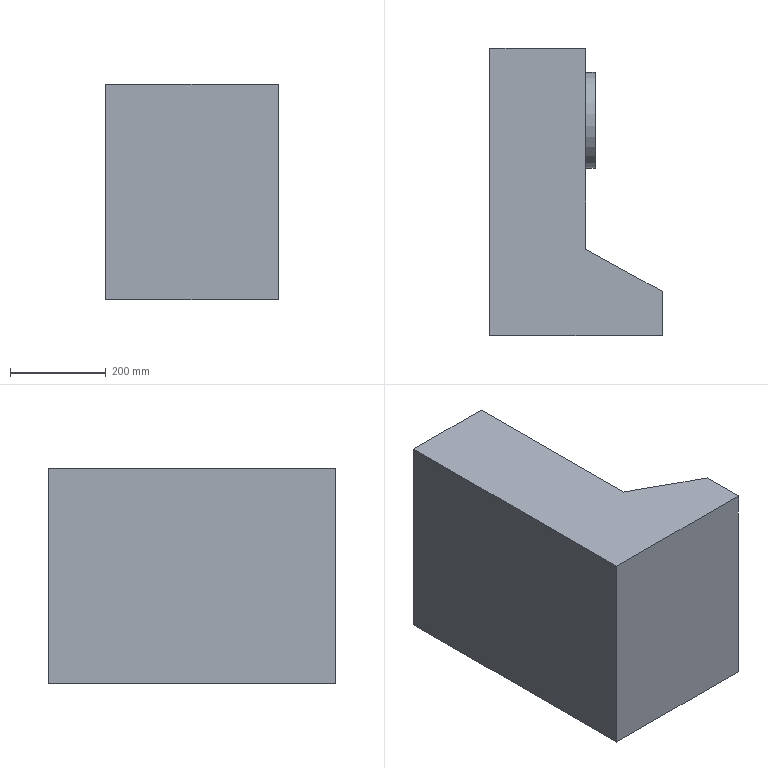Part | SolidWorks | features ICE 3, Extrusion 1 | 1 solid | 11 faces | box 360 x 600 x 450 mm | volume 64420319 mm3 | plane 9 | cylinder 2 | commonest cylinder face diameters 200 x2
STEP:
#1=CARTESIAN_POINT('',(220.,250.,0.));
#2=VERTEX_POINT('',#1);
#3=CARTESIAN_POINT('',(220.,50.,0.));
#4=VERTEX_POINT('',#3);
#5=CARTESIAN_POINT('',(220.,150.,0.));
#6=DIRECTION('',(1.,0.,0.));
#7=DIRECTION('',(0.,1.,0.));
#8=AXIS2_PLACEMENT_3D('',#5,#6,#7);
#9=CIRCLE('',#8,100.);
#10=EDGE_CURVE('',#2,#4,#9,.T.);
#11=ORIENTED_EDGE('',*,*,#10,.F.);
#12=CARTESIAN_POINT('',(200.,250.,0.));
#13=VERTEX_POINT('',#12);
#14=CARTESIAN_POINT('',(220.,250.,0.));
#15=DIRECTION('',(-1.,0.,0.));
#16=VECTOR('',#15,1000.);
#17=LINE('',#14,#16);
#18=EDGE_CURVE('',#2,#13,#17,.T.);
#19=ORIENTED_EDGE('',*,*,#18,.T.);
#20=CARTESIAN_POINT('',(200.,50.,0.));
#21=VERTEX_POINT('',#20);
#22=CARTESIAN_POINT('',(200.,150.,0.));
#23=DIRECTION('',(1.,0.,0.));
#24=DIRECTION('',(0.,-1.,0.));
#25=AXIS2_PLACEMENT_3D('',#22,#23,#24);
#26=CIRCLE('',#25,100.);
#27=EDGE_CURVE('',#13,#21,#26,.T.);
#28=ORIENTED_EDGE('',*,*,#27,.T.);
#29=CARTESIAN_POINT('',(220.,50.,0.));
#30=DIRECTION('',(-1.,0.,0.));
#31=VECTOR('',#30,1000.);
#32=LINE('',#29,#31);
#33=EDGE_CURVE('',#4,#21,#32,.T.);
#34=ORIENTED_EDGE('',*,*,#33,.F.);
#35=EDGE_LOOP('',(#11,#19,#28,#34));
#36=FACE_OUTER_BOUND('',#35,.T.);
#37=CARTESIAN_POINT('',(220.,150.,0.));
#38=DIRECTION('',(-1.,0.,0.));
#39=DIRECTION('',(0.,-1.,0.));
#40=AXIS2_PLACEMENT_3D('',#37,#38,#39);
#41=CYLINDRICAL_SURFACE('',#40,100.);
#42=ADVANCED_FACE('',(#36),#41,.T.);
#43=CARTESIAN_POINT('',(360.,-300.,-225.));
#44=VERTEX_POINT('',#43);
#45=CARTESIAN_POINT('',(360.,-208.,-225.));
#46=VERTEX_POINT('',#45);
#47=CARTESIAN_POINT('',(360.,300.,-225.));
#48=DIRECTION('',(0.,1.,0.));
#49=VECTOR('',#48,1000.);
#50=LINE('',#47,#49);
#51=EDGE_CURVE('',#44,#46,#50,.T.);
#52=ORIENTED_EDGE('',*,*,#51,.F.);
#53=CARTESIAN_POINT('',(0.,-300.,-225.));
#54=VERTEX_POINT('',#53);
#55=CARTESIAN_POINT('',(400.,-300.,-225.));
#56=DIRECTION('',(-1.,0.,0.));
#57=VECTOR('',#56,1000.);
#58=LINE('',#55,#57);
#59=EDGE_CURVE('',#44,#54,#58,.T.);
#60=ORIENTED_EDGE('',*,*,#59,.T.);
#61=CARTESIAN_POINT('',(0.,300.,-225.));
#62=VERTEX_POINT('',#61);
#63=CARTESIAN_POINT('',(0.,300.,-225.));
#64=DIRECTION('',(0.,1.,0.));
#65=VECTOR('',#64,1000.);
#66=LINE('',#63,#65);
#67=EDGE_CURVE('',#54,#62,#66,.T.);
#68=ORIENTED_EDGE('',*,*,#67,.T.);
#69=CARTESIAN_POINT('',(200.,300.,-225.));
#70=VERTEX_POINT('',#69);
#71=CARTESIAN_POINT('',(400.,300.,-225.));
#72=DIRECTION('',(-1.,0.,0.));
#73=VECTOR('',#72,1000.);
#74=LINE('',#71,#73);
#75=EDGE_CURVE('',#70,#62,#74,.T.);
#76=ORIENTED_EDGE('',*,*,#75,.F.);
#77=CARTESIAN_POINT('',(200.,-120.,-225.));
#78=VERTEX_POINT('',#77);
#79=CARTESIAN_POINT('',(200.,300.,-225.));
#80=DIRECTION('',(0.,-1.,0.));
#81=VECTOR('',#80,1000.);
#82=LINE('',#79,#81);
#83=EDGE_CURVE('',#70,#78,#82,.T.);
#84=ORIENTED_EDGE('',*,*,#83,.T.);
#85=CARTESIAN_POINT('',(176.2,-106.91,-225.));
#86=DIRECTION('',(0.8762,-0.4819,0.));
#87=VECTOR('',#86,1000.);
#88=LINE('',#85,#87);
#89=EDGE_CURVE('',#78,#46,#88,.T.);
#90=ORIENTED_EDGE('',*,*,#89,.T.);
#91=EDGE_LOOP('',(#52,#60,#68,#76,#84,#90));
#92=FACE_OUTER_BOUND('',#91,.T.);
#93=CARTESIAN_POINT('',(400.,300.,-225.));
#94=DIRECTION('',(0.,0.,1.));
#95=DIRECTION('',(1.,0.,0.));
#96=AXIS2_PLACEMENT_3D('',#93,#94,#95);
#97=PLANE('',#96);
#98=ADVANCED_FACE('',(#92),#97,.F.);
#99=CARTESIAN_POINT('',(360.,-208.,225.));
#100=VERTEX_POINT('',#99);
#101=CARTESIAN_POINT('',(360.,-300.,225.));
#102=VERTEX_POINT('',#101);
#103=CARTESIAN_POINT('',(360.,300.,225.));
#104=DIRECTION('',(0.,-1.,0.));
#105=VECTOR('',#104,1000.);
#106=LINE('',#103,#105);
#107=EDGE_CURVE('',#100,#102,#106,.T.);
#108=ORIENTED_EDGE('',*,*,#107,.F.);
#109=CARTESIAN_POINT('',(200.,-120.,225.));
#110=VERTEX_POINT('',#109);
#111=CARTESIAN_POINT('',(200.,-120.,225.));
#112=DIRECTION('',(0.8762,-0.4819,0.));
#113=VECTOR('',#112,1000.);
#114=LINE('',#111,#113);
#115=EDGE_CURVE('',#110,#100,#114,.T.);
#116=ORIENTED_EDGE('',*,*,#115,.F.);
#117=CARTESIAN_POINT('',(200.,300.,225.));
#118=VERTEX_POINT('',#117);
#119=CARTESIAN_POINT('',(200.,300.,225.));
#120=DIRECTION('',(0.,-1.,0.));
#121=VECTOR('',#120,1000.);
#122=LINE('',#119,#121);
#123=EDGE_CURVE('',#118,#110,#122,.T.);
#124=ORIENTED_EDGE('',*,*,#123,.F.);
#125=CARTESIAN_POINT('',(0.,300.,225.));
#126=VERTEX_POINT('',#125);
#127=CARTESIAN_POINT('',(400.,300.,225.));
#128=DIRECTION('',(-1.,0.,0.));
#129=VECTOR('',#128,1000.);
#130=LINE('',#127,#129);
#131=EDGE_CURVE('',#118,#126,#130,.T.);
#132=ORIENTED_EDGE('',*,*,#131,.T.);
#133=CARTESIAN_POINT('',(0.,-300.,225.));
#134=VERTEX_POINT('',#133);
#135=CARTESIAN_POINT('',(0.,300.,225.));
#136=DIRECTION('',(0.,-1.,0.));
#137=VECTOR('',#136,1000.);
#138=LINE('',#135,#137);
#139=EDGE_CURVE('',#126,#134,#138,.T.);
#140=ORIENTED_EDGE('',*,*,#139,.T.);
#141=CARTESIAN_POINT('',(400.,-300.,225.));
#142=DIRECTION('',(-1.,0.,0.));
#143=VECTOR('',#142,1000.);
#144=LINE('',#141,#143);
#145=EDGE_CURVE('',#102,#134,#144,.T.);
#146=ORIENTED_EDGE('',*,*,#145,.F.);
#147=EDGE_LOOP('',(#108,#116,#124,#132,#140,#146));
#148=FACE_OUTER_BOUND('',#147,.T.);
#149=CARTESIAN_POINT('',(400.,300.,225.));
#150=DIRECTION('',(0.,0.,-1.));
#151=DIRECTION('',(0.,1.,0.));
#152=AXIS2_PLACEMENT_3D('',#149,#150,#151);
#153=PLANE('',#152);
#154=ADVANCED_FACE('',(#148),#153,.F.);
#155=CARTESIAN_POINT('',(360.,-300.,225.));
#156=DIRECTION('',(0.,0.,-1.));
#157=VECTOR('',#156,1000.);
#158=LINE('',#155,#157);
#159=EDGE_CURVE('',#102,#44,#158,.T.);
#160=ORIENTED_EDGE('',*,*,#159,.F.);
#161=ORIENTED_EDGE('',*,*,#145,.T.);
#162=CARTESIAN_POINT('',(0.,-300.,225.));
#163=DIRECTION('',(0.,0.,-1.));
#164=VECTOR('',#163,1000.);
#165=LINE('',#162,#164);
#166=EDGE_CURVE('',#134,#54,#165,.T.);
#167=ORIENTED_EDGE('',*,*,#166,.T.);
#168=ORIENTED_EDGE('',*,*,#59,.F.);
#169=EDGE_LOOP('',(#160,#161,#167,#168));
#170=FACE_OUTER_BOUND('',#169,.T.);
#171=CARTESIAN_POINT('',(400.,-300.,225.));
#172=DIRECTION('',(0.,1.,0.));
#173=DIRECTION('',(0.,0.,1.));
#174=AXIS2_PLACEMENT_3D('',#171,#172,#173);
#175=PLANE('',#174);
#176=ADVANCED_FACE('',(#170),#175,.F.);
#177=CARTESIAN_POINT('',(360.,-208.,-2175.));
#178=DIRECTION('',(0.,0.,1.));
#179=VECTOR('',#178,1000.);
#180=LINE('',#177,#179);
#181=EDGE_CURVE('',#46,#100,#180,.T.);
#182=ORIENTED_EDGE('',*,*,#181,.F.);
#183=ORIENTED_EDGE('',*,*,#89,.F.);
#184=CARTESIAN_POINT('',(200.,-120.,-2175.));
#185=DIRECTION('',(0.,0.,1.));
#186=VECTOR('',#185,1000.);
#187=LINE('',#184,#186);
#188=EDGE_CURVE('',#78,#110,#187,.T.);
#189=ORIENTED_EDGE('',*,*,#188,.T.);
#190=ORIENTED_EDGE('',*,*,#115,.T.);
#191=EDGE_LOOP('',(#182,#183,#189,#190));
#192=FACE_OUTER_BOUND('',#191,.T.);
#193=CARTESIAN_POINT('',(200.,-120.,-2175.));
#194=DIRECTION('',(-0.4819,-0.8762,0.));
#195=DIRECTION('',(0.8762,-0.4819,0.));
#196=AXIS2_PLACEMENT_3D('',#193,#194,#195);
#197=PLANE('',#196);
#198=ADVANCED_FACE('',(#192),#197,.F.);
#199=ORIENTED_EDGE('',*,*,#131,.F.);
#200=CARTESIAN_POINT('',(200.,300.,-2175.));
#201=DIRECTION('',(0.,0.,1.));
#202=VECTOR('',#201,1000.);
#203=LINE('',#200,#202);
#204=EDGE_CURVE('',#70,#118,#203,.T.);
#205=ORIENTED_EDGE('',*,*,#204,.F.);
#206=ORIENTED_EDGE('',*,*,#75,.T.);
#207=CARTESIAN_POINT('',(0.,300.,225.));
#208=DIRECTION('',(0.,0.,1.));
#209=VECTOR('',#208,1000.);
#210=LINE('',#207,#209);
#211=EDGE_CURVE('',#62,#126,#210,.T.);
#212=ORIENTED_EDGE('',*,*,#211,.T.);
#213=EDGE_LOOP('',(#199,#205,#206,#212));
#214=FACE_OUTER_BOUND('',#213,.T.);
#215=CARTESIAN_POINT('',(400.,300.,225.));
#216=DIRECTION('',(0.,-1.,0.));
#217=DIRECTION('',(0.,0.,-1.));
#218=AXIS2_PLACEMENT_3D('',#215,#216,#217);
#219=PLANE('',#218);
#220=ADVANCED_FACE('',(#214),#219,.F.);
#221=ORIENTED_EDGE('',*,*,#67,.F.);
#222=ORIENTED_EDGE('',*,*,#166,.F.);
#223=ORIENTED_EDGE('',*,*,#139,.F.);
#224=ORIENTED_EDGE('',*,*,#211,.F.);
#225=EDGE_LOOP('',(#221,#222,#223,#224));
#226=FACE_OUTER_BOUND('',#225,.T.);
#227=CARTESIAN_POINT('',(0.,0.,0.));
#228=DIRECTION('',(1.,0.,0.));
#229=DIRECTION('',(0.,0.,-1.));
#230=AXIS2_PLACEMENT_3D('',#227,#228,#229);
#231=PLANE('',#230);
#232=ADVANCED_FACE('',(#226),#231,.F.);
#233=CARTESIAN_POINT('',(200.,150.,0.));
#234=DIRECTION('',(1.,0.,0.));
#235=DIRECTION('',(0.,-1.,0.));
#236=AXIS2_PLACEMENT_3D('',#233,#234,#235);
#237=CIRCLE('',#236,100.);
#238=EDGE_CURVE('',#21,#13,#237,.T.);
#239=ORIENTED_EDGE('',*,*,#238,.F.);
#240=ORIENTED_EDGE('',*,*,#27,.F.);
#241=EDGE_LOOP('',(#239,#240));
#242=FACE_BOUND('',#241,.T.);
#243=ORIENTED_EDGE('',*,*,#204,.T.);
#244=ORIENTED_EDGE('',*,*,#123,.T.);
#245=ORIENTED_EDGE('',*,*,#188,.F.);
#246=ORIENTED_EDGE('',*,*,#83,.F.);
#247=EDGE_LOOP('',(#243,#244,#245,#246));
#248=FACE_OUTER_BOUND('',#247,.T.);
#249=CARTESIAN_POINT('',(200.,300.,-2175.));
#250=DIRECTION('',(-1.,0.,0.));
#251=DIRECTION('',(0.,-1.,0.));
#252=AXIS2_PLACEMENT_3D('',#249,#250,#251);
#253=PLANE('',#252);
#254=ADVANCED_FACE('',(#242,#248),#253,.F.);
#255=ORIENTED_EDGE('',*,*,#159,.T.);
#256=ORIENTED_EDGE('',*,*,#51,.T.);
#257=ORIENTED_EDGE('',*,*,#181,.T.);
#258=ORIENTED_EDGE('',*,*,#107,.T.);
#259=EDGE_LOOP('',(#255,#256,#257,#258));
#260=FACE_OUTER_BOUND('',#259,.T.);
#261=CARTESIAN_POINT('',(360.,0.,0.));
#262=DIRECTION('',(1.,0.,0.));
#263=DIRECTION('',(0.,0.,-1.));
#264=AXIS2_PLACEMENT_3D('',#261,#262,#263);
#265=PLANE('',#264);
#266=ADVANCED_FACE('',(#260),#265,.T.);
#267=ORIENTED_EDGE('',*,*,#18,.F.);
#268=CARTESIAN_POINT('',(220.,150.,0.));
#269=DIRECTION('',(1.,0.,0.));
#270=DIRECTION('',(0.,1.,0.));
#271=AXIS2_PLACEMENT_3D('',#268,#269,#270);
#272=CIRCLE('',#271,100.);
#273=EDGE_CURVE('',#4,#2,#272,.T.);
#274=ORIENTED_EDGE('',*,*,#273,.F.);
#275=ORIENTED_EDGE('',*,*,#33,.T.);
#276=ORIENTED_EDGE('',*,*,#238,.T.);
#277=EDGE_LOOP('',(#267,#274,#275,#276));
#278=FACE_OUTER_BOUND('',#277,.T.);
#279=CARTESIAN_POINT('',(220.,150.,0.));
#280=DIRECTION('',(-1.,0.,0.));
#281=DIRECTION('',(0.,-1.,0.));
#282=AXIS2_PLACEMENT_3D('',#279,#280,#281);
#283=CYLINDRICAL_SURFACE('',#282,100.);
#284=ADVANCED_FACE('',(#278),#283,.T.);
#285=ORIENTED_EDGE('',*,*,#273,.T.);
#286=ORIENTED_EDGE('',*,*,#10,.T.);
#287=EDGE_LOOP('',(#285,#286));
#288=FACE_OUTER_BOUND('',#287,.T.);
#289=CARTESIAN_POINT('',(220.,150.,0.));
#290=DIRECTION('',(1.,0.,0.));
#291=DIRECTION('',(0.,1.,0.));
#292=AXIS2_PLACEMENT_3D('',#289,#290,#291);
#293=PLANE('',#292);
#294=ADVANCED_FACE('',(#288),#293,.T.);
#295=CLOSED_SHELL('',(#42,#98,#154,#176,#198,#220,#232,#254,#266,#284,#294));
#296=MANIFOLD_SOLID_BREP('',#295);
#297=CARTESIAN_POINT('',(0.,0.,0.));
#298=DIRECTION('',(0.,0.,1.));
#299=DIRECTION('',(1.,0.,0.));
#300=AXIS2_PLACEMENT_3D('',#297,#298,#299);
#301=(LENGTH_UNIT()NAMED_UNIT(*)SI_UNIT(.MILLI.,.METRE.));
#302=UNCERTAINTY_MEASURE_WITH_UNIT(LENGTH_MEASURE(0.00001),#301,'','');
#303=(NAMED_UNIT(*)PLANE_ANGLE_UNIT()SI_UNIT($,.RADIAN.));
#304=(NAMED_UNIT(*)SI_UNIT($,.STERADIAN.)SOLID_ANGLE_UNIT());
#305=(GEOMETRIC_REPRESENTATION_CONTEXT(3)GLOBAL_UNCERTAINTY_ASSIGNED_CONTEXT((#302))GLOBAL_UNIT_ASSIGNED_CONTEXT((#301,#303,#304))REPRESENTATION_CONTEXT('',''));
#306=ADVANCED_BREP_SHAPE_REPRESENTATION('',(#296,#300),#305);